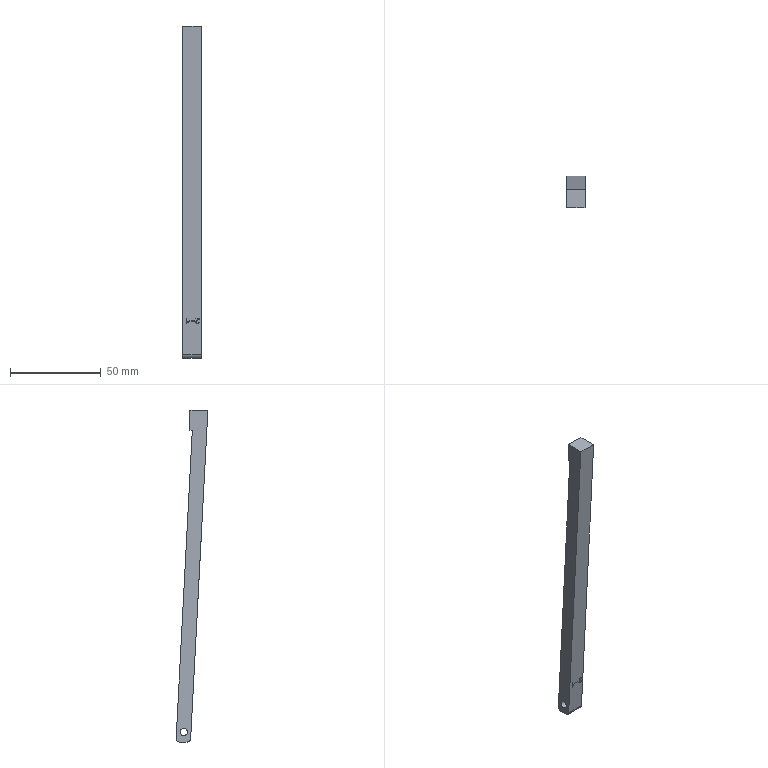Part | STEP file | solid 27 | 1 solid | 46 faces | box 10 x 17.491 x 182.939 mm | volume 14658 mm3 | plane 37 | cylinder 5 | other 4 | commonest cylinder face diameters 4 x3 1.005 x1 6922 x1